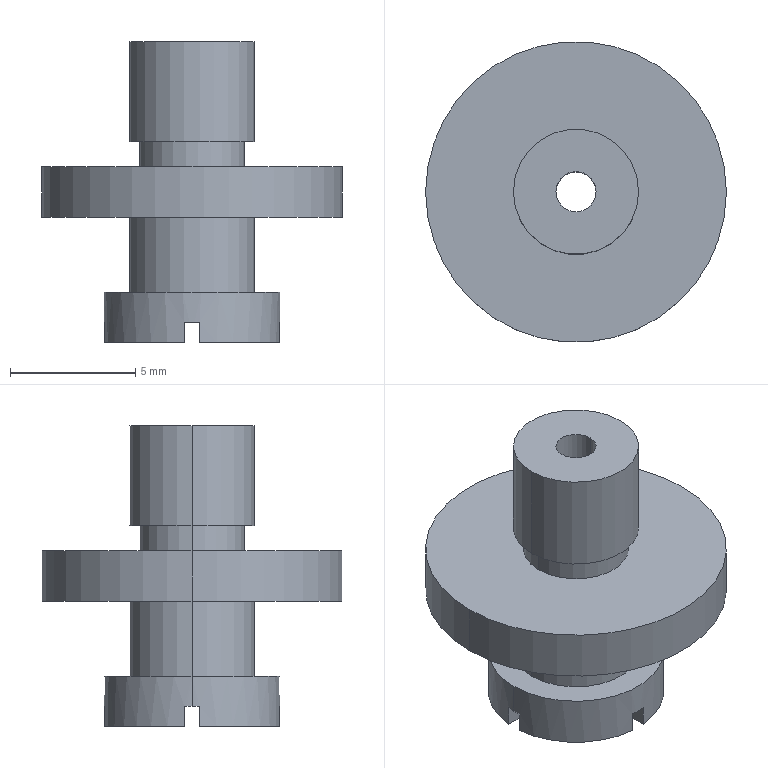Part | STEP file | 0-19 Suction cup screw rod | 1 solid | 33 faces | box 12 x 12 x 12 mm | volume 425.123 mm3 | plane 21 | cylinder 12 | commonest cylinder face diameters 5 x4 1.6 x2 4.2 x2 7 x2 12 x2